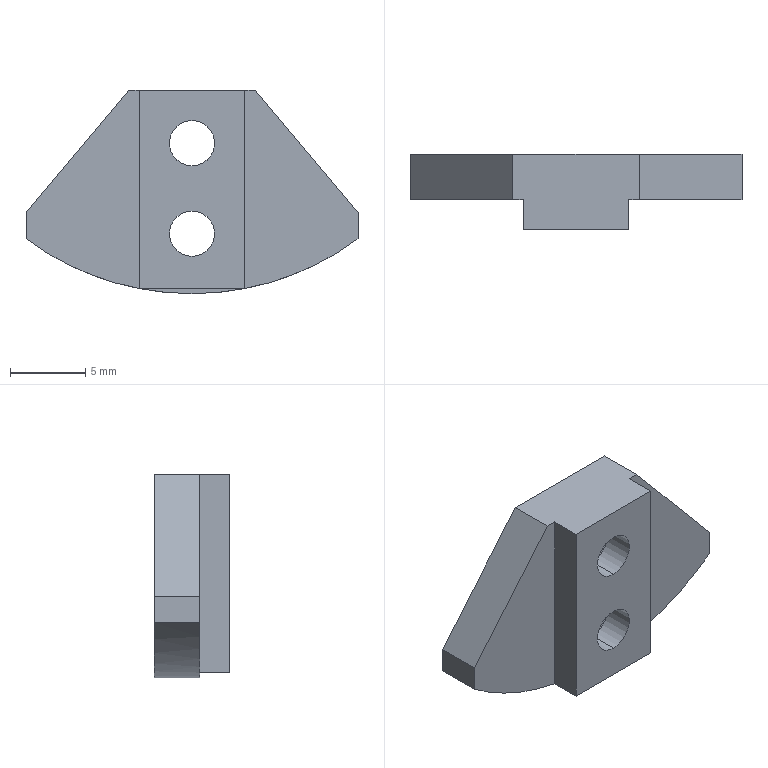Part | STEP file | Guide wheel mechanism revised.sldasm-Part-398 | 1 solid | 24 faces | box 22 x 5 x 13.47 mm | volume 660.101 mm3 | plane 15 | cylinder 9 | commonest cylinder face diameters 3 x4 5.5 x4 36.941 x1
STEP:
#1=CARTESIAN_POINT('',(0.,2.,-11.25));
#2=VERTEX_POINT('',#1);
#3=CARTESIAN_POINT('',(0.,2.,-5.75));
#4=VERTEX_POINT('',#3);
#5=CARTESIAN_POINT('',(0.,2.,-8.5));
#6=DIRECTION('',(0.,1.,0.));
#7=DIRECTION('',(0.,0.,1.));
#8=AXIS2_PLACEMENT_3D('',#5,#6,#7);
#9=CIRCLE('',#8,2.75);
#10=EDGE_CURVE('',#2,#4,#9,.T.);
#11=ORIENTED_EDGE('',*,*,#10,.F.);
#12=CARTESIAN_POINT('',(0.,5.,-11.25));
#13=VERTEX_POINT('',#12);
#14=CARTESIAN_POINT('',(0.,2.,-11.25));
#15=DIRECTION('',(0.,1.,0.));
#16=VECTOR('',#15,1000.);
#17=LINE('',#14,#16);
#18=EDGE_CURVE('',#2,#13,#17,.T.);
#19=ORIENTED_EDGE('',*,*,#18,.T.);
#20=CARTESIAN_POINT('',(0.,5.,-5.75));
#21=VERTEX_POINT('',#20);
#22=CARTESIAN_POINT('',(0.,5.,-8.5));
#23=DIRECTION('',(0.,1.,0.));
#24=DIRECTION('',(0.,0.,1.));
#25=AXIS2_PLACEMENT_3D('',#22,#23,#24);
#26=CIRCLE('',#25,2.75);
#27=EDGE_CURVE('',#13,#21,#26,.T.);
#28=ORIENTED_EDGE('',*,*,#27,.T.);
#29=CARTESIAN_POINT('',(0.,2.,-5.75));
#30=DIRECTION('',(0.,1.,0.));
#31=VECTOR('',#30,1000.);
#32=LINE('',#29,#31);
#33=EDGE_CURVE('',#4,#21,#32,.T.);
#34=ORIENTED_EDGE('',*,*,#33,.F.);
#35=EDGE_LOOP('',(#11,#19,#28,#34));
#36=FACE_OUTER_BOUND('',#35,.T.);
#37=CARTESIAN_POINT('',(0.,2.,-8.5));
#38=DIRECTION('',(0.,1.,0.));
#39=DIRECTION('',(0.,0.,1.));
#40=AXIS2_PLACEMENT_3D('',#37,#38,#39);
#41=CYLINDRICAL_SURFACE('',#40,2.75);
#42=ADVANCED_FACE('',(#36),#41,.F.);
#43=CARTESIAN_POINT('',(0.,2.,-17.25));
#44=VERTEX_POINT('',#43);
#45=CARTESIAN_POINT('',(0.,2.,-11.75));
#46=VERTEX_POINT('',#45);
#47=CARTESIAN_POINT('',(0.,2.,-14.5));
#48=DIRECTION('',(0.,1.,0.));
#49=DIRECTION('',(0.,0.,1.));
#50=AXIS2_PLACEMENT_3D('',#47,#48,#49);
#51=CIRCLE('',#50,2.75);
#52=EDGE_CURVE('',#44,#46,#51,.T.);
#53=ORIENTED_EDGE('',*,*,#52,.F.);
#54=CARTESIAN_POINT('',(0.,5.,-17.25));
#55=VERTEX_POINT('',#54);
#56=CARTESIAN_POINT('',(0.,2.,-17.25));
#57=DIRECTION('',(0.,1.,0.));
#58=VECTOR('',#57,1000.);
#59=LINE('',#56,#58);
#60=EDGE_CURVE('',#44,#55,#59,.T.);
#61=ORIENTED_EDGE('',*,*,#60,.T.);
#62=CARTESIAN_POINT('',(0.,5.,-11.75));
#63=VERTEX_POINT('',#62);
#64=CARTESIAN_POINT('',(0.,5.,-14.5));
#65=DIRECTION('',(0.,1.,0.));
#66=DIRECTION('',(0.,0.,1.));
#67=AXIS2_PLACEMENT_3D('',#64,#65,#66);
#68=CIRCLE('',#67,2.75);
#69=EDGE_CURVE('',#55,#63,#68,.T.);
#70=ORIENTED_EDGE('',*,*,#69,.T.);
#71=CARTESIAN_POINT('',(0.,2.,-11.75));
#72=DIRECTION('',(0.,1.,0.));
#73=VECTOR('',#72,1000.);
#74=LINE('',#71,#73);
#75=EDGE_CURVE('',#46,#63,#74,.T.);
#76=ORIENTED_EDGE('',*,*,#75,.F.);
#77=EDGE_LOOP('',(#53,#61,#70,#76));
#78=FACE_OUTER_BOUND('',#77,.T.);
#79=CARTESIAN_POINT('',(0.,2.,-14.5));
#80=DIRECTION('',(0.,1.,0.));
#81=DIRECTION('',(0.,0.,1.));
#82=AXIS2_PLACEMENT_3D('',#79,#80,#81);
#83=CYLINDRICAL_SURFACE('',#82,2.75);
#84=ADVANCED_FACE('',(#78),#83,.F.);
#85=CARTESIAN_POINT('',(0.,0.,-16.));
#86=VERTEX_POINT('',#85);
#87=CARTESIAN_POINT('',(0.,0.,-13.));
#88=VERTEX_POINT('',#87);
#89=CARTESIAN_POINT('',(0.,0.,-14.5));
#90=DIRECTION('',(0.,1.,0.));
#91=DIRECTION('',(0.,0.,1.));
#92=AXIS2_PLACEMENT_3D('',#89,#90,#91);
#93=CIRCLE('',#92,1.5);
#94=EDGE_CURVE('',#86,#88,#93,.T.);
#95=ORIENTED_EDGE('',*,*,#94,.F.);
#96=CARTESIAN_POINT('',(0.,2.,-16.));
#97=VERTEX_POINT('',#96);
#98=CARTESIAN_POINT('',(0.,0.,-16.));
#99=DIRECTION('',(0.,1.,0.));
#100=VECTOR('',#99,1000.);
#101=LINE('',#98,#100);
#102=EDGE_CURVE('',#86,#97,#101,.T.);
#103=ORIENTED_EDGE('',*,*,#102,.T.);
#104=CARTESIAN_POINT('',(0.,2.,-13.));
#105=VERTEX_POINT('',#104);
#106=CARTESIAN_POINT('',(0.,2.,-14.5));
#107=DIRECTION('',(0.,-1.,0.));
#108=DIRECTION('',(0.,0.,1.));
#109=AXIS2_PLACEMENT_3D('',#106,#107,#108);
#110=CIRCLE('',#109,1.5);
#111=EDGE_CURVE('',#105,#97,#110,.T.);
#112=ORIENTED_EDGE('',*,*,#111,.F.);
#113=CARTESIAN_POINT('',(0.,0.,-13.));
#114=DIRECTION('',(0.,1.,0.));
#115=VECTOR('',#114,1000.);
#116=LINE('',#113,#115);
#117=EDGE_CURVE('',#88,#105,#116,.T.);
#118=ORIENTED_EDGE('',*,*,#117,.F.);
#119=EDGE_LOOP('',(#95,#103,#112,#118));
#120=FACE_OUTER_BOUND('',#119,.T.);
#121=CARTESIAN_POINT('',(0.,0.,-14.5));
#122=DIRECTION('',(0.,1.,0.));
#123=DIRECTION('',(0.,0.,1.));
#124=AXIS2_PLACEMENT_3D('',#121,#122,#123);
#125=CYLINDRICAL_SURFACE('',#124,1.5);
#126=ADVANCED_FACE('',(#120),#125,.F.);
#127=CARTESIAN_POINT('',(0.,0.,-10.));
#128=VERTEX_POINT('',#127);
#129=CARTESIAN_POINT('',(0.,0.,-7.));
#130=VERTEX_POINT('',#129);
#131=CARTESIAN_POINT('',(0.,0.,-8.5));
#132=DIRECTION('',(0.,1.,0.));
#133=DIRECTION('',(0.,0.,1.));
#134=AXIS2_PLACEMENT_3D('',#131,#132,#133);
#135=CIRCLE('',#134,1.5);
#136=EDGE_CURVE('',#128,#130,#135,.T.);
#137=ORIENTED_EDGE('',*,*,#136,.F.);
#138=CARTESIAN_POINT('',(0.,2.,-10.));
#139=VERTEX_POINT('',#138);
#140=CARTESIAN_POINT('',(0.,0.,-10.));
#141=DIRECTION('',(0.,1.,0.));
#142=VECTOR('',#141,1000.);
#143=LINE('',#140,#142);
#144=EDGE_CURVE('',#128,#139,#143,.T.);
#145=ORIENTED_EDGE('',*,*,#144,.T.);
#146=CARTESIAN_POINT('',(0.,2.,-7.));
#147=VERTEX_POINT('',#146);
#148=CARTESIAN_POINT('',(0.,2.,-8.5));
#149=DIRECTION('',(0.,-1.,0.));
#150=DIRECTION('',(0.,0.,1.));
#151=AXIS2_PLACEMENT_3D('',#148,#149,#150);
#152=CIRCLE('',#151,1.5);
#153=EDGE_CURVE('',#147,#139,#152,.T.);
#154=ORIENTED_EDGE('',*,*,#153,.F.);
#155=CARTESIAN_POINT('',(0.,0.,-7.));
#156=DIRECTION('',(0.,1.,0.));
#157=VECTOR('',#156,1000.);
#158=LINE('',#155,#157);
#159=EDGE_CURVE('',#130,#147,#158,.T.);
#160=ORIENTED_EDGE('',*,*,#159,.F.);
#161=EDGE_LOOP('',(#137,#145,#154,#160));
#162=FACE_OUTER_BOUND('',#161,.T.);
#163=CARTESIAN_POINT('',(0.,0.,-8.5));
#164=DIRECTION('',(0.,1.,0.));
#165=DIRECTION('',(0.,0.,1.));
#166=AXIS2_PLACEMENT_3D('',#163,#164,#165);
#167=CYLINDRICAL_SURFACE('',#166,1.5);
#168=ADVANCED_FACE('',(#162),#167,.F.);
#169=CARTESIAN_POINT('',(3.5,2.,-5.));
#170=VERTEX_POINT('',#169);
#171=CARTESIAN_POINT('',(3.5,2.,-18.136));
#172=VERTEX_POINT('',#171);
#173=CARTESIAN_POINT('',(3.5,2.,-18.136));
#174=DIRECTION('',(0.,0.,-1.));
#175=VECTOR('',#174,1000.);
#176=LINE('',#173,#175);
#177=EDGE_CURVE('',#170,#172,#176,.T.);
#178=ORIENTED_EDGE('',*,*,#177,.F.);
#179=CARTESIAN_POINT('',(3.5,0.,-5.));
#180=VERTEX_POINT('',#179);
#181=CARTESIAN_POINT('',(3.5,5.,-5.));
#182=DIRECTION('',(0.,-1.,0.));
#183=VECTOR('',#182,1000.);
#184=LINE('',#181,#183);
#185=EDGE_CURVE('',#170,#180,#184,.T.);
#186=ORIENTED_EDGE('',*,*,#185,.T.);
#187=CARTESIAN_POINT('',(3.5,0.,-18.136));
#188=VERTEX_POINT('',#187);
#189=CARTESIAN_POINT('',(3.5,0.,-18.136));
#190=DIRECTION('',(0.,0.,-1.));
#191=VECTOR('',#190,1000.);
#192=LINE('',#189,#191);
#193=EDGE_CURVE('',#180,#188,#192,.T.);
#194=ORIENTED_EDGE('',*,*,#193,.T.);
#195=CARTESIAN_POINT('',(3.5,5.,-18.136));
#196=DIRECTION('',(0.,-1.,0.));
#197=VECTOR('',#196,1000.);
#198=LINE('',#195,#197);
#199=EDGE_CURVE('',#172,#188,#198,.T.);
#200=ORIENTED_EDGE('',*,*,#199,.F.);
#201=EDGE_LOOP('',(#178,#186,#194,#200));
#202=FACE_OUTER_BOUND('',#201,.T.);
#203=CARTESIAN_POINT('',(3.5,5.,-18.136));
#204=DIRECTION('',(-1.,0.,0.));
#205=DIRECTION('',(0.,0.,1.));
#206=AXIS2_PLACEMENT_3D('',#203,#204,#205);
#207=PLANE('',#206);
#208=ADVANCED_FACE('',(#202),#207,.F.);
#209=CARTESIAN_POINT('',(-3.5,2.,-18.136));
#210=VERTEX_POINT('',#209);
#211=CARTESIAN_POINT('',(-3.5,2.,-18.136));
#212=DIRECTION('',(-1.,0.,0.));
#213=VECTOR('',#212,1000.);
#214=LINE('',#211,#213);
#215=EDGE_CURVE('',#172,#210,#214,.T.);
#216=ORIENTED_EDGE('',*,*,#215,.F.);
#217=ORIENTED_EDGE('',*,*,#199,.T.);
#218=CARTESIAN_POINT('',(-3.5,0.,-18.136));
#219=VERTEX_POINT('',#218);
#220=CARTESIAN_POINT('',(-3.5,0.,-18.136));
#221=DIRECTION('',(-1.,0.,0.));
#222=VECTOR('',#221,1000.);
#223=LINE('',#220,#222);
#224=EDGE_CURVE('',#188,#219,#223,.T.);
#225=ORIENTED_EDGE('',*,*,#224,.T.);
#226=CARTESIAN_POINT('',(-3.5,5.,-18.136));
#227=DIRECTION('',(0.,-1.,0.));
#228=VECTOR('',#227,1000.);
#229=LINE('',#226,#228);
#230=EDGE_CURVE('',#210,#219,#229,.T.);
#231=ORIENTED_EDGE('',*,*,#230,.F.);
#232=EDGE_LOOP('',(#216,#217,#225,#231));
#233=FACE_OUTER_BOUND('',#232,.T.);
#234=CARTESIAN_POINT('',(-3.5,5.,-18.136));
#235=DIRECTION('',(0.,0.,1.));
#236=DIRECTION('',(1.,0.,0.));
#237=AXIS2_PLACEMENT_3D('',#234,#235,#236);
#238=PLANE('',#237);
#239=ADVANCED_FACE('',(#233),#238,.F.);
#240=CARTESIAN_POINT('',(-3.5,2.,-5.));
#241=VERTEX_POINT('',#240);
#242=CARTESIAN_POINT('',(-3.5,2.,-6.5));
#243=DIRECTION('',(0.,0.,1.));
#244=VECTOR('',#243,1000.);
#245=LINE('',#242,#244);
#246=EDGE_CURVE('',#210,#241,#245,.T.);
#247=ORIENTED_EDGE('',*,*,#246,.F.);
#248=ORIENTED_EDGE('',*,*,#230,.T.);
#249=CARTESIAN_POINT('',(-3.5,0.,-5.));
#250=VERTEX_POINT('',#249);
#251=CARTESIAN_POINT('',(-3.5,0.,-6.5));
#252=DIRECTION('',(0.,0.,1.));
#253=VECTOR('',#252,1000.);
#254=LINE('',#251,#253);
#255=EDGE_CURVE('',#219,#250,#254,.T.);
#256=ORIENTED_EDGE('',*,*,#255,.T.);
#257=CARTESIAN_POINT('',(-3.5,5.,-5.));
#258=DIRECTION('',(0.,-1.,0.));
#259=VECTOR('',#258,1000.);
#260=LINE('',#257,#259);
#261=EDGE_CURVE('',#241,#250,#260,.T.);
#262=ORIENTED_EDGE('',*,*,#261,.F.);
#263=EDGE_LOOP('',(#247,#248,#256,#262));
#264=FACE_OUTER_BOUND('',#263,.T.);
#265=CARTESIAN_POINT('',(-3.5,5.,-6.5));
#266=DIRECTION('',(1.,0.,0.));
#267=DIRECTION('',(0.,0.,-1.));
#268=AXIS2_PLACEMENT_3D('',#265,#266,#267);
#269=PLANE('',#268);
#270=ADVANCED_FACE('',(#264),#269,.F.);
#271=ORIENTED_EDGE('',*,*,#144,.F.);
#272=CARTESIAN_POINT('',(0.,0.,-8.5));
#273=DIRECTION('',(0.,1.,0.));
#274=DIRECTION('',(0.,0.,1.));
#275=AXIS2_PLACEMENT_3D('',#272,#273,#274);
#276=CIRCLE('',#275,1.5);
#277=EDGE_CURVE('',#130,#128,#276,.T.);
#278=ORIENTED_EDGE('',*,*,#277,.F.);
#279=ORIENTED_EDGE('',*,*,#159,.T.);
#280=CARTESIAN_POINT('',(0.,2.,-8.5));
#281=DIRECTION('',(0.,-1.,0.));
#282=DIRECTION('',(0.,0.,1.));
#283=AXIS2_PLACEMENT_3D('',#280,#281,#282);
#284=CIRCLE('',#283,1.5);
#285=EDGE_CURVE('',#139,#147,#284,.T.);
#286=ORIENTED_EDGE('',*,*,#285,.F.);
#287=EDGE_LOOP('',(#271,#278,#279,#286));
#288=FACE_OUTER_BOUND('',#287,.T.);
#289=CARTESIAN_POINT('',(0.,0.,-8.5));
#290=DIRECTION('',(0.,1.,0.));
#291=DIRECTION('',(0.,0.,1.));
#292=AXIS2_PLACEMENT_3D('',#289,#290,#291);
#293=CYLINDRICAL_SURFACE('',#292,1.5);
#294=ADVANCED_FACE('',(#288),#293,.F.);
#295=ORIENTED_EDGE('',*,*,#102,.F.);
#296=CARTESIAN_POINT('',(0.,0.,-14.5));
#297=DIRECTION('',(0.,1.,0.));
#298=DIRECTION('',(0.,0.,1.));
#299=AXIS2_PLACEMENT_3D('',#296,#297,#298);
#300=CIRCLE('',#299,1.5);
#301=EDGE_CURVE('',#88,#86,#300,.T.);
#302=ORIENTED_EDGE('',*,*,#301,.F.);
#303=ORIENTED_EDGE('',*,*,#117,.T.);
#304=CARTESIAN_POINT('',(0.,2.,-14.5));
#305=DIRECTION('',(0.,-1.,0.));
#306=DIRECTION('',(0.,0.,1.));
#307=AXIS2_PLACEMENT_3D('',#304,#305,#306);
#308=CIRCLE('',#307,1.5);
#309=EDGE_CURVE('',#97,#105,#308,.T.);
#310=ORIENTED_EDGE('',*,*,#309,.F.);
#311=EDGE_LOOP('',(#295,#302,#303,#310));
#312=FACE_OUTER_BOUND('',#311,.T.);
#313=CARTESIAN_POINT('',(0.,0.,-14.5));
#314=DIRECTION('',(0.,1.,0.));
#315=DIRECTION('',(0.,0.,1.));
#316=AXIS2_PLACEMENT_3D('',#313,#314,#315);
#317=CYLINDRICAL_SURFACE('',#316,1.5);
#318=ADVANCED_FACE('',(#312),#317,.F.);
#319=CARTESIAN_POINT('',(3.5,0.,-5.));
#320=DIRECTION('',(1.,0.,0.));
#321=VECTOR('',#320,1000.);
#322=LINE('',#319,#321);
#323=EDGE_CURVE('',#250,#180,#322,.T.);
#324=ORIENTED_EDGE('',*,*,#323,.T.);
#325=ORIENTED_EDGE('',*,*,#185,.F.);
#326=CARTESIAN_POINT('',(4.195,2.,-5.));
#327=VERTEX_POINT('',#326);
#328=CARTESIAN_POINT('',(3.5,2.,-5.));
#329=DIRECTION('',(1.,0.,0.));
#330=VECTOR('',#329,1000.);
#331=LINE('',#328,#330);
#332=EDGE_CURVE('',#170,#327,#331,.T.);
#333=ORIENTED_EDGE('',*,*,#332,.T.);
#334=CARTESIAN_POINT('',(4.195,5.,-5.));
#335=VERTEX_POINT('',#334);
#336=CARTESIAN_POINT('',(4.195,2.,-5.));
#337=DIRECTION('',(0.,1.,0.));
#338=VECTOR('',#337,1000.);
#339=LINE('',#336,#338);
#340=EDGE_CURVE('',#327,#335,#339,.T.);
#341=ORIENTED_EDGE('',*,*,#340,.T.);
#342=CARTESIAN_POINT('',(-4.195,5.,-5.));
#343=VERTEX_POINT('',#342);
#344=CARTESIAN_POINT('',(3.5,5.,-5.));
#345=DIRECTION('',(1.,0.,0.));
#346=VECTOR('',#345,1000.);
#347=LINE('',#344,#346);
#348=EDGE_CURVE('',#343,#335,#347,.T.);
#349=ORIENTED_EDGE('',*,*,#348,.F.);
#350=CARTESIAN_POINT('',(-4.195,2.,-5.));
#351=VERTEX_POINT('',#350);
#352=CARTESIAN_POINT('',(-4.195,2.,-5.));
#353=DIRECTION('',(0.,1.,0.));
#354=VECTOR('',#353,1000.);
#355=LINE('',#352,#354);
#356=EDGE_CURVE('',#351,#343,#355,.T.);
#357=ORIENTED_EDGE('',*,*,#356,.F.);
#358=CARTESIAN_POINT('',(-3.5,2.,-5.));
#359=DIRECTION('',(1.,0.,0.));
#360=VECTOR('',#359,1000.);
#361=LINE('',#358,#360);
#362=EDGE_CURVE('',#351,#241,#361,.T.);
#363=ORIENTED_EDGE('',*,*,#362,.T.);
#364=ORIENTED_EDGE('',*,*,#261,.T.);
#365=EDGE_LOOP('',(#324,#325,#333,#341,#349,#357,#363,#364));
#366=FACE_OUTER_BOUND('',#365,.T.);
#367=CARTESIAN_POINT('',(3.5,5.,-5.));
#368=DIRECTION('',(0.,0.,-1.));
#369=DIRECTION('',(-1.,0.,0.));
#370=AXIS2_PLACEMENT_3D('',#367,#368,#369);
#371=PLANE('',#370);
#372=ADVANCED_FACE('',(#366),#371,.F.);
#373=CARTESIAN_POINT('',(11.,5.,-14.838));
#374=VERTEX_POINT('',#373);
#375=CARTESIAN_POINT('',(-11.,5.,-14.838));
#376=VERTEX_POINT('',#375);
#377=CARTESIAN_POINT('',(0.,5.,0.));
#378=DIRECTION('',(0.,1.,0.));
#379=DIRECTION('',(0.,0.,1.));
#380=AXIS2_PLACEMENT_3D('',#377,#378,#379);
#381=CIRCLE('',#380,18.47);
#382=EDGE_CURVE('',#374,#376,#381,.T.);
#383=ORIENTED_EDGE('',*,*,#382,.T.);
#384=CARTESIAN_POINT('',(-11.,5.,-13.109));
#385=VERTEX_POINT('',#384);
#386=CARTESIAN_POINT('',(-11.,5.,-13.109));
#387=DIRECTION('',(0.,0.,1.));
#388=VECTOR('',#387,1000.);
#389=LINE('',#386,#388);
#390=EDGE_CURVE('',#376,#385,#389,.T.);
#391=ORIENTED_EDGE('',*,*,#390,.T.);
#392=CARTESIAN_POINT('',(-4.195,5.,-5.));
#393=DIRECTION('',(0.6428,0.,0.766));
#394=VECTOR('',#393,1000.);
#395=LINE('',#392,#394);
#396=EDGE_CURVE('',#385,#343,#395,.T.);
#397=ORIENTED_EDGE('',*,*,#396,.T.);
#398=ORIENTED_EDGE('',*,*,#348,.T.);
#399=CARTESIAN_POINT('',(11.,5.,-13.109));
#400=VERTEX_POINT('',#399);
#401=CARTESIAN_POINT('',(4.195,5.,-5.));
#402=DIRECTION('',(0.6428,0.,-0.766));
#403=VECTOR('',#402,1000.);
#404=LINE('',#401,#403);
#405=EDGE_CURVE('',#335,#400,#404,.T.);
#406=ORIENTED_EDGE('',*,*,#405,.T.);
#407=CARTESIAN_POINT('',(11.,5.,-13.109));
#408=DIRECTION('',(0.,0.,-1.));
#409=VECTOR('',#408,1000.);
#410=LINE('',#407,#409);
#411=EDGE_CURVE('',#400,#374,#410,.T.);
#412=ORIENTED_EDGE('',*,*,#411,.T.);
#413=EDGE_LOOP('',(#383,#391,#397,#398,#406,#412));
#414=FACE_OUTER_BOUND('',#413,.T.);
#415=CARTESIAN_POINT('',(0.,5.,-8.5));
#416=DIRECTION('',(0.,1.,0.));
#417=DIRECTION('',(0.,0.,1.));
#418=AXIS2_PLACEMENT_3D('',#415,#416,#417);
#419=CIRCLE('',#418,2.75);
#420=EDGE_CURVE('',#21,#13,#419,.T.);
#421=ORIENTED_EDGE('',*,*,#420,.F.);
#422=ORIENTED_EDGE('',*,*,#27,.F.);
#423=EDGE_LOOP('',(#421,#422));
#424=FACE_BOUND('',#423,.T.);
#425=CARTESIAN_POINT('',(0.,5.,-14.5));
#426=DIRECTION('',(0.,1.,0.));
#427=DIRECTION('',(0.,0.,1.));
#428=AXIS2_PLACEMENT_3D('',#425,#426,#427);
#429=CIRCLE('',#428,2.75);
#430=EDGE_CURVE('',#63,#55,#429,.T.);
#431=ORIENTED_EDGE('',*,*,#430,.F.);
#432=ORIENTED_EDGE('',*,*,#69,.F.);
#433=EDGE_LOOP('',(#431,#432));
#434=FACE_BOUND('',#433,.T.);
#435=CARTESIAN_POINT('',(0.,5.,0.));
#436=DIRECTION('',(0.,-1.,0.));
#437=DIRECTION('',(0.,0.,-1.));
#438=AXIS2_PLACEMENT_3D('',#435,#436,#437);
#439=PLANE('',#438);
#440=ADVANCED_FACE('',(#414,#424,#434),#439,.F.);
#441=ORIENTED_EDGE('',*,*,#277,.T.);
#442=ORIENTED_EDGE('',*,*,#136,.T.);
#443=EDGE_LOOP('',(#441,#442));
#444=FACE_BOUND('',#443,.T.);
#445=ORIENTED_EDGE('',*,*,#301,.T.);
#446=ORIENTED_EDGE('',*,*,#94,.T.);
#447=EDGE_LOOP('',(#445,#446));
#448=FACE_BOUND('',#447,.T.);
#449=ORIENTED_EDGE('',*,*,#323,.F.);
#450=ORIENTED_EDGE('',*,*,#255,.F.);
#451=ORIENTED_EDGE('',*,*,#224,.F.);
#452=ORIENTED_EDGE('',*,*,#193,.F.);
#453=EDGE_LOOP('',(#449,#450,#451,#452));
#454=FACE_OUTER_BOUND('',#453,.T.);
#455=CARTESIAN_POINT('',(0.,0.,0.));
#456=DIRECTION('',(0.,-1.,0.));
#457=DIRECTION('',(0.,0.,-1.));
#458=AXIS2_PLACEMENT_3D('',#455,#456,#457);
#459=PLANE('',#458);
#460=ADVANCED_FACE('',(#444,#448,#454),#459,.T.);
#461=CARTESIAN_POINT('',(0.,2.,-14.5));
#462=DIRECTION('',(0.,1.,0.));
#463=DIRECTION('',(0.,0.,1.));
#464=AXIS2_PLACEMENT_3D('',#461,#462,#463);
#465=CIRCLE('',#464,2.75);
#466=EDGE_CURVE('',#46,#44,#465,.T.);
#467=ORIENTED_EDGE('',*,*,#466,.T.);
#468=ORIENTED_EDGE('',*,*,#52,.T.);
#469=EDGE_LOOP('',(#467,#468));
#470=FACE_OUTER_BOUND('',#469,.T.);
#471=ORIENTED_EDGE('',*,*,#111,.T.);
#472=ORIENTED_EDGE('',*,*,#309,.T.);
#473=EDGE_LOOP('',(#471,#472));
#474=FACE_BOUND('',#473,.T.);
#475=CARTESIAN_POINT('',(0.,2.,-14.5));
#476=DIRECTION('',(0.,1.,0.));
#477=DIRECTION('',(0.,0.,1.));
#478=AXIS2_PLACEMENT_3D('',#475,#476,#477);
#479=PLANE('',#478);
#480=ADVANCED_FACE('',(#470,#474),#479,.T.);
#481=ORIENTED_EDGE('',*,*,#60,.F.);
#482=ORIENTED_EDGE('',*,*,#466,.F.);
#483=ORIENTED_EDGE('',*,*,#75,.T.);
#484=ORIENTED_EDGE('',*,*,#430,.T.);
#485=EDGE_LOOP('',(#481,#482,#483,#484));
#486=FACE_OUTER_BOUND('',#485,.T.);
#487=CARTESIAN_POINT('',(0.,2.,-14.5));
#488=DIRECTION('',(0.,1.,0.));
#489=DIRECTION('',(0.,0.,1.));
#490=AXIS2_PLACEMENT_3D('',#487,#488,#489);
#491=CYLINDRICAL_SURFACE('',#490,2.75);
#492=ADVANCED_FACE('',(#486),#491,.F.);
#493=CARTESIAN_POINT('',(0.,2.,-8.5));
#494=DIRECTION('',(0.,1.,0.));
#495=DIRECTION('',(0.,0.,1.));
#496=AXIS2_PLACEMENT_3D('',#493,#494,#495);
#497=CIRCLE('',#496,2.75);
#498=EDGE_CURVE('',#4,#2,#497,.T.);
#499=ORIENTED_EDGE('',*,*,#498,.T.);
#500=ORIENTED_EDGE('',*,*,#10,.T.);
#501=EDGE_LOOP('',(#499,#500));
#502=FACE_OUTER_BOUND('',#501,.T.);
#503=ORIENTED_EDGE('',*,*,#153,.T.);
#504=ORIENTED_EDGE('',*,*,#285,.T.);
#505=EDGE_LOOP('',(#503,#504));
#506=FACE_BOUND('',#505,.T.);
#507=CARTESIAN_POINT('',(0.,2.,-8.5));
#508=DIRECTION('',(0.,1.,0.));
#509=DIRECTION('',(0.,0.,1.));
#510=AXIS2_PLACEMENT_3D('',#507,#508,#509);
#511=PLANE('',#510);
#512=ADVANCED_FACE('',(#502,#506),#511,.T.);
#513=ORIENTED_EDGE('',*,*,#18,.F.);
#514=ORIENTED_EDGE('',*,*,#498,.F.);
#515=ORIENTED_EDGE('',*,*,#33,.T.);
#516=ORIENTED_EDGE('',*,*,#420,.T.);
#517=EDGE_LOOP('',(#513,#514,#515,#516));
#518=FACE_OUTER_BOUND('',#517,.T.);
#519=CARTESIAN_POINT('',(0.,2.,-8.5));
#520=DIRECTION('',(0.,1.,0.));
#521=DIRECTION('',(0.,0.,1.));
#522=AXIS2_PLACEMENT_3D('',#519,#520,#521);
#523=CYLINDRICAL_SURFACE('',#522,2.75);
#524=ADVANCED_FACE('',(#518),#523,.F.);
#525=ORIENTED_EDGE('',*,*,#332,.F.);
#526=ORIENTED_EDGE('',*,*,#177,.T.);
#527=CARTESIAN_POINT('',(11.,2.,-14.838));
#528=VERTEX_POINT('',#527);
#529=CARTESIAN_POINT('',(0.,2.,0.));
#530=DIRECTION('',(0.,1.,0.));
#531=DIRECTION('',(0.,0.,1.));
#532=AXIS2_PLACEMENT_3D('',#529,#530,#531);
#533=CIRCLE('',#532,18.47);
#534=EDGE_CURVE('',#528,#172,#533,.T.);
#535=ORIENTED_EDGE('',*,*,#534,.F.);
#536=CARTESIAN_POINT('',(11.,2.,-13.109));
#537=VERTEX_POINT('',#536);
#538=CARTESIAN_POINT('',(11.,2.,-13.109));
#539=DIRECTION('',(0.,0.,-1.));
#540=VECTOR('',#539,1000.);
#541=LINE('',#538,#540);
#542=EDGE_CURVE('',#537,#528,#541,.T.);
#543=ORIENTED_EDGE('',*,*,#542,.F.);
#544=CARTESIAN_POINT('',(4.195,2.,-5.));
#545=DIRECTION('',(0.6428,0.,-0.766));
#546=VECTOR('',#545,1000.);
#547=LINE('',#544,#546);
#548=EDGE_CURVE('',#327,#537,#547,.T.);
#549=ORIENTED_EDGE('',*,*,#548,.F.);
#550=EDGE_LOOP('',(#525,#526,#535,#543,#549));
#551=FACE_OUTER_BOUND('',#550,.T.);
#552=CARTESIAN_POINT('',(0.,2.,0.));
#553=DIRECTION('',(0.,1.,0.));
#554=DIRECTION('',(0.,0.,1.));
#555=AXIS2_PLACEMENT_3D('',#552,#553,#554);
#556=PLANE('',#555);
#557=ADVANCED_FACE('',(#551),#556,.F.);
#558=CARTESIAN_POINT('',(0.,2.,0.));
#559=DIRECTION('',(0.,1.,0.));
#560=DIRECTION('',(0.,0.,1.));
#561=AXIS2_PLACEMENT_3D('',#558,#559,#560);
#562=CIRCLE('',#561,18.47);
#563=EDGE_CURVE('',#172,#210,#562,.T.);
#564=ORIENTED_EDGE('',*,*,#563,.F.);
#565=ORIENTED_EDGE('',*,*,#215,.T.);
#566=EDGE_LOOP('',(#564,#565));
#567=FACE_OUTER_BOUND('',#566,.T.);
#568=CARTESIAN_POINT('',(0.,2.,0.));
#569=DIRECTION('',(0.,1.,0.));
#570=DIRECTION('',(0.,0.,1.));
#571=AXIS2_PLACEMENT_3D('',#568,#569,#570);
#572=PLANE('',#571);
#573=ADVANCED_FACE('',(#567),#572,.F.);
#574=CARTESIAN_POINT('',(-11.,2.,-14.838));
#575=VERTEX_POINT('',#574);
#576=CARTESIAN_POINT('',(0.,2.,0.));
#577=DIRECTION('',(0.,1.,0.));
#578=DIRECTION('',(0.,0.,1.));
#579=AXIS2_PLACEMENT_3D('',#576,#577,#578);
#580=CIRCLE('',#579,18.47);
#581=EDGE_CURVE('',#210,#575,#580,.T.);
#582=ORIENTED_EDGE('',*,*,#581,.F.);
#583=ORIENTED_EDGE('',*,*,#246,.T.);
#584=ORIENTED_EDGE('',*,*,#362,.F.);
#585=CARTESIAN_POINT('',(-11.,2.,-13.109));
#586=VERTEX_POINT('',#585);
#587=CARTESIAN_POINT('',(-4.195,2.,-5.));
#588=DIRECTION('',(0.6428,0.,0.766));
#589=VECTOR('',#588,1000.);
#590=LINE('',#587,#589);
#591=EDGE_CURVE('',#586,#351,#590,.T.);
#592=ORIENTED_EDGE('',*,*,#591,.F.);
#593=CARTESIAN_POINT('',(-11.,2.,-13.109));
#594=DIRECTION('',(0.,0.,1.));
#595=VECTOR('',#594,1000.);
#596=LINE('',#593,#595);
#597=EDGE_CURVE('',#575,#586,#596,.T.);
#598=ORIENTED_EDGE('',*,*,#597,.F.);
#599=EDGE_LOOP('',(#582,#583,#584,#592,#598));
#600=FACE_OUTER_BOUND('',#599,.T.);
#601=CARTESIAN_POINT('',(0.,2.,0.));
#602=DIRECTION('',(0.,1.,0.));
#603=DIRECTION('',(0.,0.,1.));
#604=AXIS2_PLACEMENT_3D('',#601,#602,#603);
#605=PLANE('',#604);
#606=ADVANCED_FACE('',(#600),#605,.F.);
#607=CARTESIAN_POINT('',(-11.,2.,-14.838));
#608=DIRECTION('',(0.,1.,0.));
#609=VECTOR('',#608,1000.);
#610=LINE('',#607,#609);
#611=EDGE_CURVE('',#575,#376,#610,.T.);
#612=ORIENTED_EDGE('',*,*,#611,.T.);
#613=ORIENTED_EDGE('',*,*,#382,.F.);
#614=CARTESIAN_POINT('',(11.,2.,-14.838));
#615=DIRECTION('',(0.,1.,0.));
#616=VECTOR('',#615,1000.);
#617=LINE('',#614,#616);
#618=EDGE_CURVE('',#528,#374,#617,.T.);
#619=ORIENTED_EDGE('',*,*,#618,.F.);
#620=ORIENTED_EDGE('',*,*,#534,.T.);
#621=ORIENTED_EDGE('',*,*,#563,.T.);
#622=ORIENTED_EDGE('',*,*,#581,.T.);
#623=EDGE_LOOP('',(#612,#613,#619,#620,#621,#622));
#624=FACE_OUTER_BOUND('',#623,.T.);
#625=CARTESIAN_POINT('',(0.,2.,0.));
#626=DIRECTION('',(0.,1.,0.));
#627=DIRECTION('',(0.,0.,1.));
#628=AXIS2_PLACEMENT_3D('',#625,#626,#627);
#629=CYLINDRICAL_SURFACE('',#628,18.47);
#630=ADVANCED_FACE('',(#624),#629,.T.);
#631=ORIENTED_EDGE('',*,*,#396,.F.);
#632=CARTESIAN_POINT('',(-11.,2.,-13.109));
#633=DIRECTION('',(0.,1.,0.));
#634=VECTOR('',#633,1000.);
#635=LINE('',#632,#634);
#636=EDGE_CURVE('',#586,#385,#635,.T.);
#637=ORIENTED_EDGE('',*,*,#636,.F.);
#638=ORIENTED_EDGE('',*,*,#591,.T.);
#639=ORIENTED_EDGE('',*,*,#356,.T.);
#640=EDGE_LOOP('',(#631,#637,#638,#639));
#641=FACE_OUTER_BOUND('',#640,.T.);
#642=CARTESIAN_POINT('',(-4.195,2.,-5.));
#643=DIRECTION('',(-0.766,0.,0.6428));
#644=DIRECTION('',(0.6428,0.,0.766));
#645=AXIS2_PLACEMENT_3D('',#642,#643,#644);
#646=PLANE('',#645);
#647=ADVANCED_FACE('',(#641),#646,.T.);
#648=ORIENTED_EDGE('',*,*,#390,.F.);
#649=ORIENTED_EDGE('',*,*,#611,.F.);
#650=ORIENTED_EDGE('',*,*,#597,.T.);
#651=ORIENTED_EDGE('',*,*,#636,.T.);
#652=EDGE_LOOP('',(#648,#649,#650,#651));
#653=FACE_OUTER_BOUND('',#652,.T.);
#654=CARTESIAN_POINT('',(-11.,2.,-13.109));
#655=DIRECTION('',(-1.,0.,0.));
#656=DIRECTION('',(0.,0.,1.));
#657=AXIS2_PLACEMENT_3D('',#654,#655,#656);
#658=PLANE('',#657);
#659=ADVANCED_FACE('',(#653),#658,.T.);
#660=ORIENTED_EDGE('',*,*,#411,.F.);
#661=CARTESIAN_POINT('',(11.,2.,-13.109));
#662=DIRECTION('',(0.,1.,0.));
#663=VECTOR('',#662,1000.);
#664=LINE('',#661,#663);
#665=EDGE_CURVE('',#537,#400,#664,.T.);
#666=ORIENTED_EDGE('',*,*,#665,.F.);
#667=ORIENTED_EDGE('',*,*,#542,.T.);
#668=ORIENTED_EDGE('',*,*,#618,.T.);
#669=EDGE_LOOP('',(#660,#666,#667,#668));
#670=FACE_OUTER_BOUND('',#669,.T.);
#671=CARTESIAN_POINT('',(11.,2.,-13.109));
#672=DIRECTION('',(1.,0.,0.));
#673=DIRECTION('',(0.,0.,-1.));
#674=AXIS2_PLACEMENT_3D('',#671,#672,#673);
#675=PLANE('',#674);
#676=ADVANCED_FACE('',(#670),#675,.T.);
#677=ORIENTED_EDGE('',*,*,#405,.F.);
#678=ORIENTED_EDGE('',*,*,#340,.F.);
#679=ORIENTED_EDGE('',*,*,#548,.T.);
#680=ORIENTED_EDGE('',*,*,#665,.T.);
#681=EDGE_LOOP('',(#677,#678,#679,#680));
#682=FACE_OUTER_BOUND('',#681,.T.);
#683=CARTESIAN_POINT('',(4.195,2.,-5.));
#684=DIRECTION('',(0.766,0.,0.6428));
#685=DIRECTION('',(0.6428,0.,-0.766));
#686=AXIS2_PLACEMENT_3D('',#683,#684,#685);
#687=PLANE('',#686);
#688=ADVANCED_FACE('',(#682),#687,.T.);
#689=CLOSED_SHELL('',(#42,#84,#126,#168,#208,#239,#270,#294,#318,#372,#440,#460,#480,#492,#512,#524,#557,#573,#606,#630,#647,#659,#676,#688));
#690=MANIFOLD_SOLID_BREP('',#689);
#691=CARTESIAN_POINT('',(0.,0.,0.));
#692=DIRECTION('',(0.,0.,1.));
#693=DIRECTION('',(1.,0.,0.));
#694=AXIS2_PLACEMENT_3D('',#691,#692,#693);
#695=(LENGTH_UNIT()NAMED_UNIT(*)SI_UNIT(.MILLI.,.METRE.));
#696=UNCERTAINTY_MEASURE_WITH_UNIT(LENGTH_MEASURE(0.00001),#695,'','');
#697=(NAMED_UNIT(*)PLANE_ANGLE_UNIT()SI_UNIT($,.RADIAN.));
#698=(NAMED_UNIT(*)SI_UNIT($,.STERADIAN.)SOLID_ANGLE_UNIT());
#699=(GEOMETRIC_REPRESENTATION_CONTEXT(3)GLOBAL_UNCERTAINTY_ASSIGNED_CONTEXT((#696))GLOBAL_UNIT_ASSIGNED_CONTEXT((#695,#697,#698))REPRESENTATION_CONTEXT('',''));
#700=ADVANCED_BREP_SHAPE_REPRESENTATION('',(#690,#694),#699);